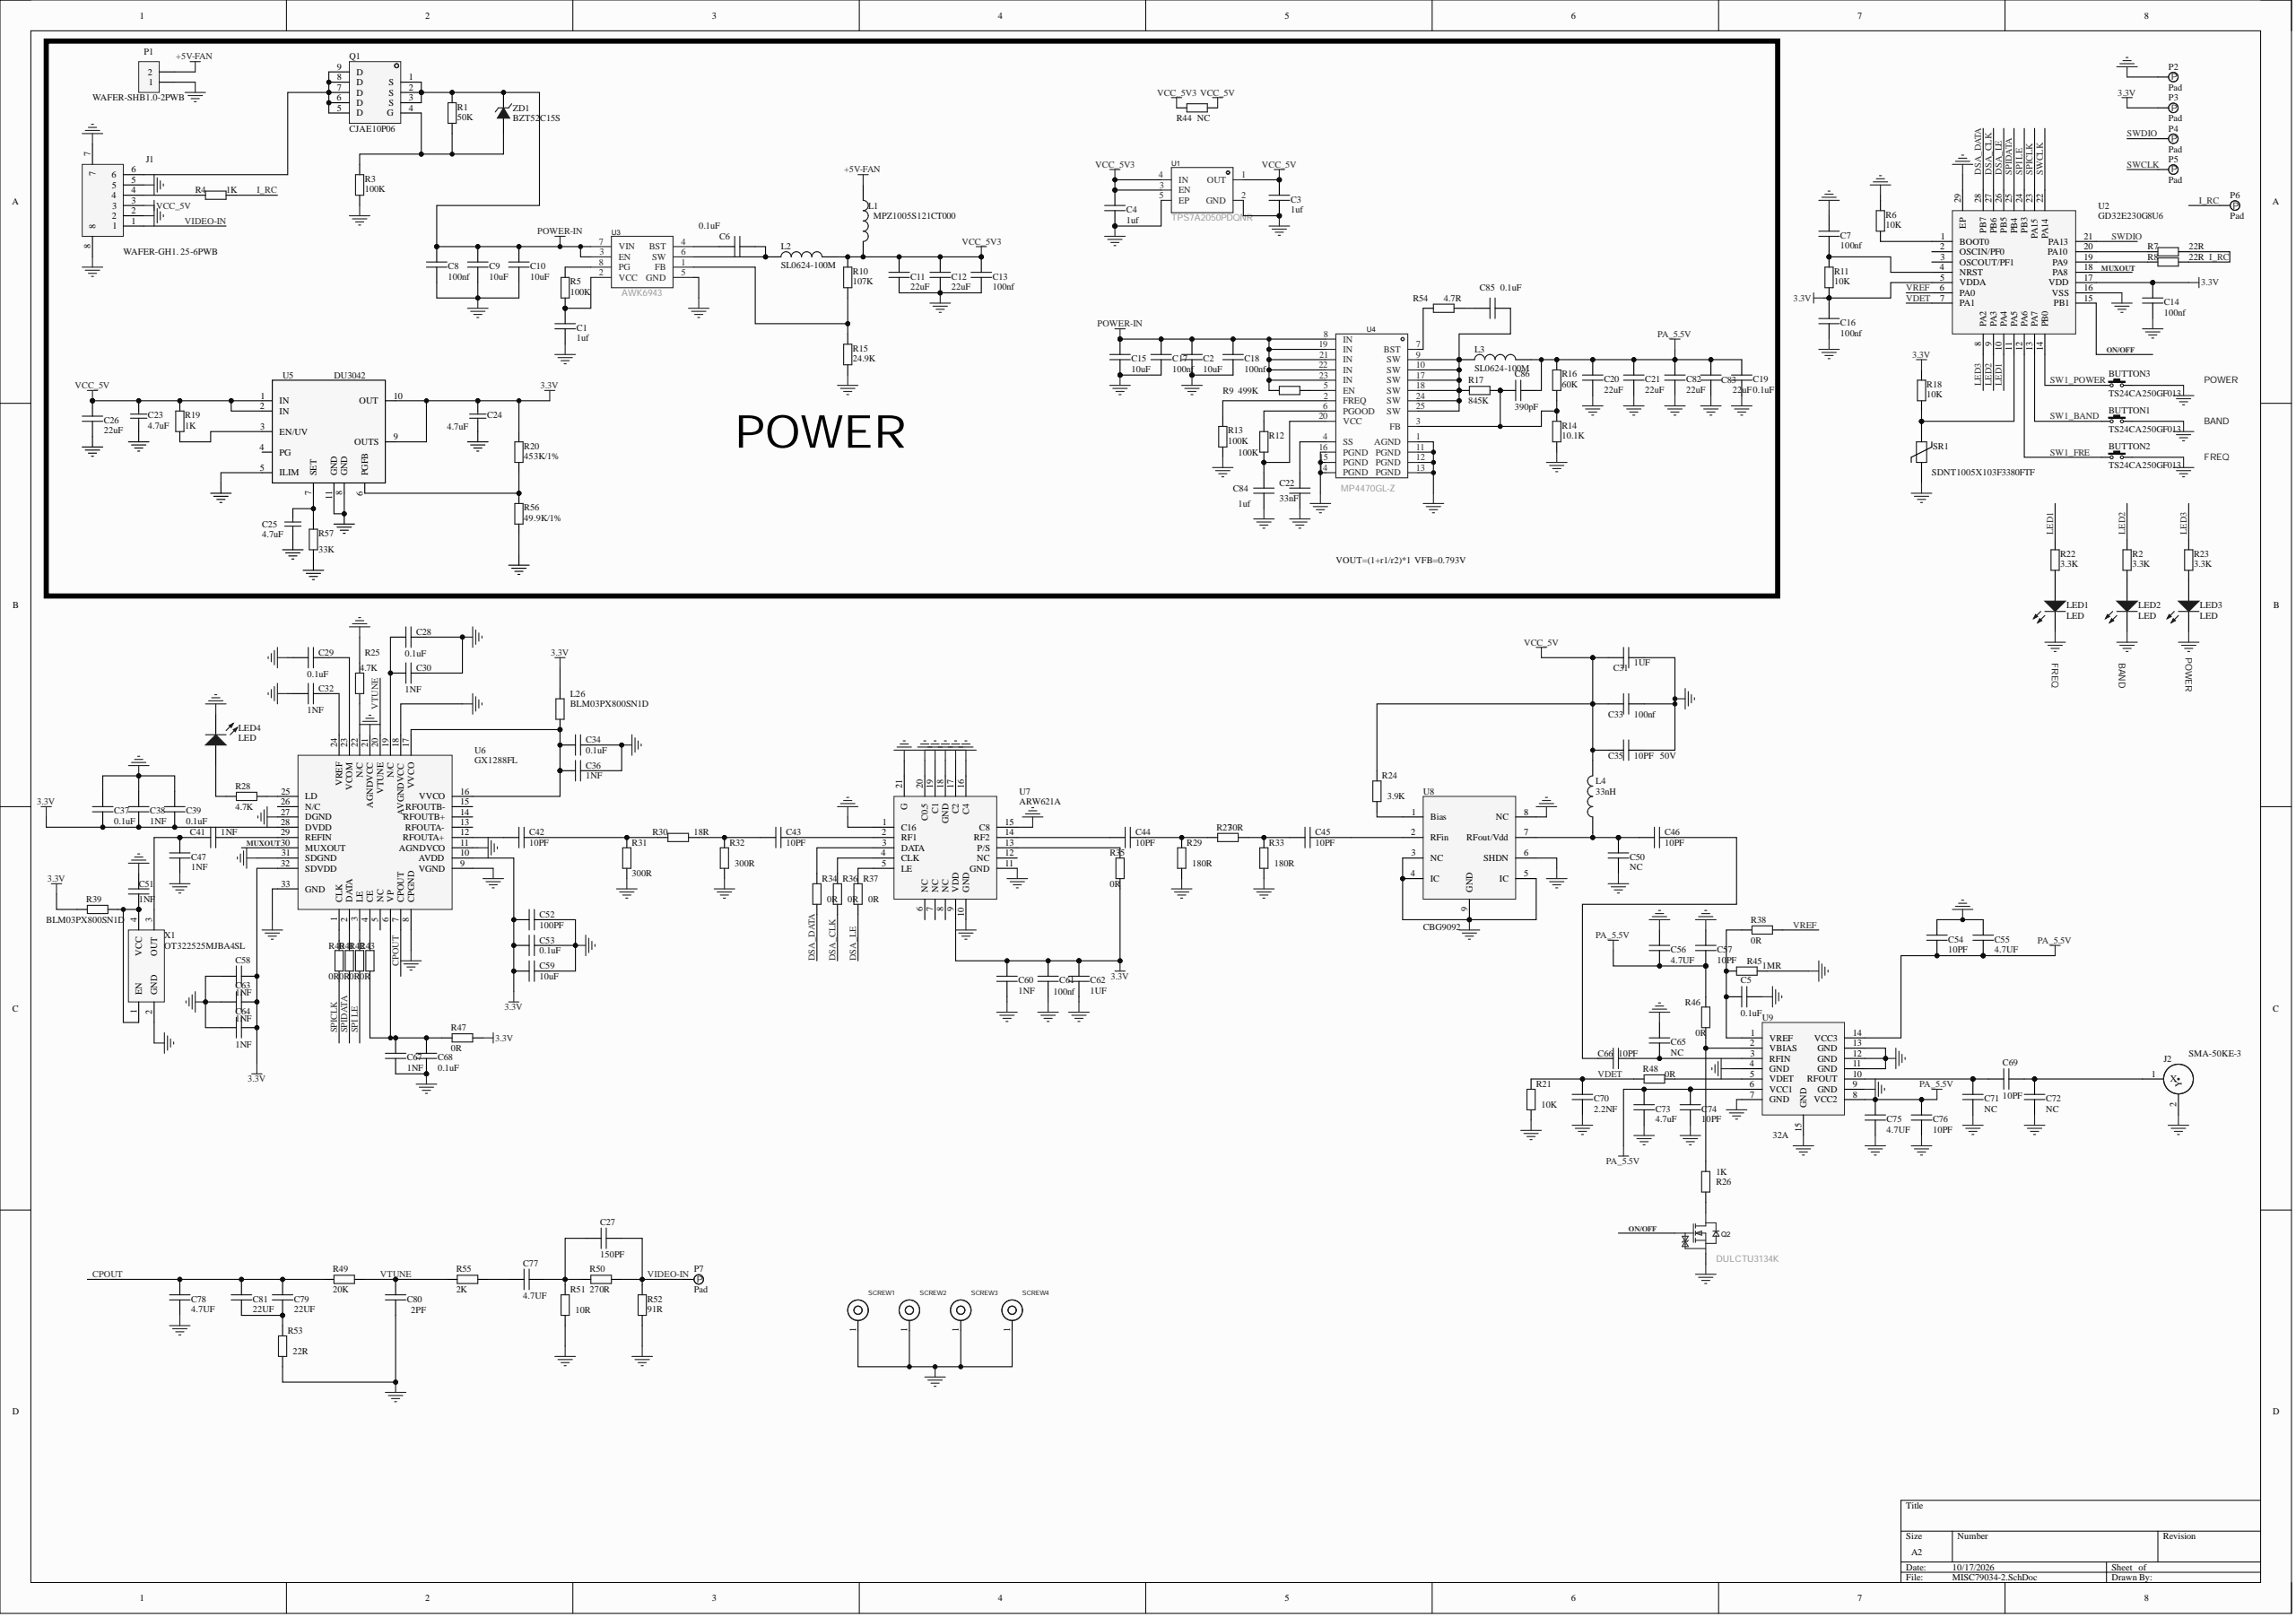Circuit board | Altium Designer | 179 parts | 97 nets
Bill of materials:
Comment,Description,Designator,Footprint,LibRef,Quantity
"TS24CA250GF013","3x6 tact switch","BUTTON1, BUTTON2, BUTTON3","SW-SMD_L4.7-W3.5-P3.35-EH","TSW 3x6","3"
"1uf","","C1, C3, C4, C84","C0603","100nf","4"
"10uF","","C2, C9, C10, C15","C0805","100nf","4"
"0.1uF","","C5, C6, C19, C85","C0402","100nf","4"
"100nf","","C7, C14, C16","C0201","100nf","3"
"100nf","","C8, C13, C17, C18, C33, C61","C0402","100nf","6"
"22uF","","C11, C12, C20, C21, C26, C82, C83","C0603","100nf","7"
"33nF","","C22","C0402","100nf","1"
"4.7uF","Chip capacitor, [NoValue]","C23, C24, C25, C55, C56, C73, C75","C0603","C, 100nf","7"
"150PF","","C27","C0402","100nf","1"
"0.1uF","","C28, C29, C34, C37, C39, C53, C68","C0201","100nf","7"
"1NF","","C30, C32, C36, C38, C41, C47, C51, C58, C63, C64, C67","C0201","100nf","11"
"1UF","","C31, C62","C0402","100nf","2"
"10PF   50V","","C35","C0402","100nf","1"
"10PF","","C42, C43, C44, C45, C46, C54, C57, C66, C69, C74, C76","C0402","100nf","11"
"NC","","C50, C65, C71, C72","C0402","100nf","4"
"100PF","","C52","C0201","100nf","1"
"10uF","","C59","C0402","100nf","1"
"1NF","","C60","C0402","100nf","1"
"2.2NF","","C70","C0402","100nf","1"
"4.7UF","","C77, C78","C0402","100nf","2"
"22UF","","C79, C81","C0402","100nf","2"
"2PF","","C80","C0402","100nf","1"
"390pF","","C86","C0402","100nf","1"
"WAFER-GH1. 25-6PWB","","J1","SMD_6P-P1.25_XUNPU_WAFER-GH1.25-6PWB","WAFER-GH1. 25-6PWB","1"
"SMA-50KE-3","","J2","SMA-FP-945G","SMA-50KE-3","1"
"MPZ1005S121CT000","Color-ring inductor","L1","L0402","L-AL","1"
"SL0624-100M","Color-ring inductor","L2, L3","IND-SMD_L7.1-W6.6","L-AL","2"
"33nH","Color-ring inductor","L4","L0402","L-AL","1"
"BLM03PX800SN1D","Chip resistor","L26, R39","L0201","R","2"
"LED","Light-emitting diode","LED1, LED2, LED3, LED4","LED0402","LED0","4"
"WAFER-SHB1.0-2PWB","2P connector","P1","SMD_2P-WAFER-SHB1.0-2PWB","Header 2","1"
"Pad","","P2, P3, P4, P5, P6, P7","pad","Pad","6"
"CJAE10P06","","Q1","DFN-8_L3.0-W3.0-P0.65-BL_G48N03D3","CJAE10P06","1"
"DULCTU3134K","","Q2","SOT-523-3_L1.6-W0.8-P0.50-LS1.6-BR-1","2N7002T_C5224243","1"
"50K","Chip resistor","R1","R0402","R","1"
"3.3K","Chip resistor","R2, R22, R23","R0402","R","3"
"100K","Chip resistor","R3, R5, R12, R13","R0402","R","4"
"1K","Chip resistor","R4, R19, R26","R0402","R","3"
"10K","Chip resistor","R6, R11, R18","R0201","R","3"
"22R","Chip resistor","R7, R8","R0201","R","2"
"499K","Chip resistor","R9","R0402","R","1"
"107K","Chip resistor","R10","R0402","R","1"
"10.1K","Chip resistor","R14","R0402","R","1"
"24.9K","Chip resistor","R15","R0402","R","1"
"60K","Chip resistor","R16","R0402","R","1"
"845K","Chip resistor","R17","R0402","R","1"
"453K/1%","Chip resistor","R20","R0402","R","1"
"10K","Chip resistor","R21","R0402","R","1"
"3.9K","Chip resistor","R24","R0402","R","1"
"4.7K","Chip resistor","R25, R28","R0201","R","2"
"30R","Chip resistor","R27","R0402","R","1"
"180R","Chip resistor","R29, R33","R0402","R","2"
"18R","Chip resistor","R30","R0402","R","1"
"300R","Chip resistor","R31, R32","R0402","R","2"
"0R","Chip resistor","R34, R35, R36, R37, R38, R46, R48","R0402","R","7"
"0R","Chip resistor","R40, R41, R42, R43, R47","R0201","R","5"
"NC","Chip resistor","R44","R0402","R","1"
"1MR","Chip resistor","R45","R0402","R","1"
"20K","Chip resistor","R49","R0402","R","1"
"270R","Chip resistor","R50","R0402","R","1"
"10R","Chip resistor","R51","R0402","R","1"
"91R","Chip resistor","R52","R0402","R","1"
"22R","Chip resistor","R53","R0402","R","1"
"4.7R","Chip resistor","R54","R1206","R","1"
"2K","Chip resistor","R55","R0402","R","1"
"49.9K/1%","Chip resistor","R56","R0402","R","1"
"33K","Chip resistor","R57","R0402","R","1"
"MARK_4","MARK Symble","SCREW1, SCREW2, SCREW3, SCREW4","M2","MARK_4","4"
"SDNT1005X103F3380FTF","","SR1","R0402","SDNT1005X103F3380FTF","1"
"TPS7A2050PDQNR","","U1","X2SON-4_L1.0-W1.0-P0.65-TL-EP","TPS7A2050PDQNR","1"
"GD32E230G8U6","","U2","QFN-28_L4.0-W4.0-P0.40-BL-EP2.8","GD32E230G8U6","1"
"AWK6943","","U3","QFN-8_L3.0-W3.0-P0.65-BL","TPS54327DDAR","1"
"MP4470GL-Z","","U4","QFN-20_L4.0-W3.0_MP9447GL","MP4470GL-Z","1"
"DU3042","No Description Available","U5","WSON-10_L3.0-W3.0-P0.50-BL-EP","DAC53202RTER","1"
"GX1288FL","","U6","QFN-32_L5.0-W5.0-P0.50","GX1288FL","1"
"ARW621A","","U7","QFN-20_L4.0-W4.0-P0.50-TL-EP2.2","ARW621A","1"
"CBG9092","","U8","CBG9092","CBG9092","1"
"32A","","U9","AU64XX","GCM3527(3.3G-3.8G)","1"
"OT322525MJBA4SL","4-pin active crystal oscillator","X1","SMD3225","XTAL-ACT-4P","1"
"BZT52C15S","5.1V/1W Zener diode","ZD1","SOD-323_L1.7-W1.3-LS2.6-RD","1N4733","1"
Netlist (Protel format):
[
BUTTON1
SW-SMD_L4.7-W3.5-P3.35-EH
TS24CA250GF013



]
[
BUTTON2
SW-SMD_L4.7-W3.5-P3.35-EH
TS24CA250GF013



]
[
BUTTON3
SW-SMD_L4.7-W3.5-P3.35-EH
TS24CA250GF013



]
[
C1
C0603
1uf



]
[
C2
C0805
10uF



]
[
C3
C0603
1uf



]
[
C4
C0603
1uf



]
[
C5
C0402
0.1uF



]
[
C6
C0402
0.1uF



]
[
C7
C0201
100nf



]
[
C8
C0402
100nf



]
[
C9
C0805
10uF



]
[
C10
C0805
10uF



]
[
C11
C0603
22uF



]
[
C12
C0603
22uF



]
[
C13
C0402
100nf



]
[
C14
C0201
100nf



]
[
C15
C0805
10uF



]
[
C16
C0201
100nf



]
[
C17
C0402
100nf



]
[
C18
C0402
100nf



]
[
C19
C0402
0.1uF



]
[
C20
C0603
22uF



]
[
C21
C0603
22uF



]
[
C22
C0402
33nF



]
[
C23
C0603
4.7uF



]
[
C24
C0603
4.7uF



]
[
C25
C0603
4.7uF



]
[
C26
C0603
22uF



]
[
C27
C0402
150PF



]
[
C28
C0201
0.1uF



]
[
C29
C0201
0.1uF



]
[
C30
C0201
1NF



]
[
C31
C0402
1UF



]
[
C32
C0201
1NF



]
[
C33
C0402
100nf



]
[
C34
C0201
0.1uF



]
[
C35
C0402
10PF   50V



]
[
C36
C0201
1NF



]
[
C37
C0201
0.1uF



]
[
C38
C0201
1NF



]
[
C39
C0201
0.1uF



]
[
C41
C0201
1NF



]
[
C42
C0402
10PF



]
[
C43
C0402
10PF



]
[
C44
C0402
10PF



]
[
C45
C0402
10PF



]
[
C46
C0402
10PF



]
[
C47
C0201
1NF



]
[
C50
C0402
NC



]
[
C51
C0201
1NF



]
[
C52
C0201
100PF



]
[
C53
C0201
0.1uF



]
[
C54
C0402
10PF



]
[
C55
C0603
4.7UF



]
[
C56
C0603
4.7UF



]
[
C57
C0402
10PF



]
[
C58
C0201
1NF



]
[
C59
C0402
10uF



]
[
C60
C0402
1NF



]
[
C61
C0402
100nf



]
[
C62
C0402
1UF



]
[
C63
C0201
1NF



]
[
C64
C0201
1NF



]
[
C65
C0402
NC



]
[
C66
C0402
10PF



]
[
C67
C0201
1NF



]
[
C68
C0201
0.1uF



]
[
C69
C0402
10PF



]
[
C70
C0402
2.2NF



]
[
C71
C0402
NC



]
[
C72
C0402
NC



]
[
C73
C0603
4.7uF



]
[
C74
C0402
10PF



]
[
C75
C0603
4.7UF



]
[
C76
C0402
10PF



]
[
C77
C0402
4.7UF



]
[
C78
C0402
4.7UF



]
[
C79
C0402
22UF



]
[
C80
C0402
2PF



]
[
C81
C0402
22UF



]
[
C82
C0603
22uF



]
[
C83
C0603
22uF



]
[
C84
C0603
1uf



]
[
C85
C0402
0.1uF



]
[
C86
C0402
390pF



]
[
J1
SMD_6P-P1.25_XUNPU_WAFER-GH1.25-6PWB
WAFER-GH1. 25-6PWB



]
[
J2
SMA-FP-945G
SMA-50KE-3



]
[
L1
L0402
MPZ1005S121CT000



]
[
L2
IND-SMD_L7.1-W6.6
SL0624-100M



]
[
L3
IND-SMD_L7.1-W6.6
SL0624-100M



]
[
L4
L0402
33nH



]
[
L26
L0201
BLM03PX800SN1D



]
[
LED1
LED0402
LED



]
[
LED2
LED0402
LED



]
[
LED3
LED0402
LED



]
[
LED4
LED0402
LED



]
[
P1
SMD_2P-WAFER-SHB1.0-2PWB
WAFER-SHB1.0-2PWB



]
[
P2
pad
Pad



]
[
P3
pad
Pad



]
[
P4
pad
Pad



]
[
P5
pad
Pad



]
[
P6
PAD
Pad



]
[
P7
PAD
Pad



]
[
Q1
DFN-8_L3.0-W3.0-P0.65-BL_G48N03D3
CJAE10P06



]
[
Q2
SOT-523-3_L1.6-W0.8-P0.50-LS1.6-BR-1
DULCTU3134K



]
[
R1
R0402
50K



]
[
R2
R0402
3.3K



]
[
R3
R0402
100K



]
[
R4
R0402
1K



]
[
R5
R0402
100K



]
[
R6
R0201
10K



]
[
R7
R0201
22R



]
[
R8
R0201
22R



]
[
R9
R0402
499K



]
[
R10
R0402
107K



]
[
R11
R0201
10K



]
[
R12
R0402
100K



]
[
R13
R0402
100K



]
[
R14
R0402
10.1K



]
[
R15
R0402
24.9K



]
[
R16
R0402
60K



]
[
R17
R0402
845K



]
[
R18
R0201
10K



]
[
R19
R0402
1K



]
[
R20
R0402
453K/1%



]
[
R21
R0402
10K



]
[
R22
R0402
3.3K



]
[
R23
R0402
3.3K



]
[
R24
R0402
3.9K



]
[
R25
R0201
4.7K



]
[
R26
R0402
1K



]
[
R27
R0402
30R



]
[
R28
R0201
4.7K



]
[
R29
R0402
180R



]
[
R30
R0402
18R



]
[
R31
R0402
300R



]
[
R32
R0402
300R



]
[
R33
R0402
180R



]
[
R34
R0402
0R



]
[
R35
R0402
0R



]
[
R36
R0402
0R



]
[
R37
R0402
0R



]
[
R38
R0402
0R



]
[
R39
L0201
BLM03PX800SN1D



]
[
R40
R0201
0R



]
[
R41
R0201
0R



]
[
R42
R0201
0R



]
[
R43
R0201
0R



]
[
R44
R0402
NC



]
[
R45
R0402
1MR



]
[
R46
R0402
0R



]
[
R47
R0201
0R



]
[
R48
R0402
0R



]
[
R49
R0402
20K



]
[
R50
R0402
270R



]
[
R51
R0402
10R



]
[
R52
R0402
91R



]
[
R53
R0402
22R



]
[
R54
R1206
4.7R



]
[
R55
R0402
2K



]
[
R56
R0402
49.9K/1%



]
[
R57
R0402
33K



]
[
SCREW1
M2
MARK_4



]
[
SCREW2
M2
MARK_4



]
[
SCREW3
M2
MARK_4



]
[
SCREW4
M2
MARK_4



]
[
SR1
R0402
SDNT1005X103F3380FTF



]
[
U1
X2SON-4_L1.0-W1.0-P0.65-TL-EP
TPS7A2050PDQNR



]
[
U2
QFN-28_L4.0-W4.0-P0.40-BL-EP2.8
GD32E230G8U6



]
[
U3
QFN-8_L3.0-W3.0-P0.65-BL
AWK6943



]
[
U4
QFN-20_L4.0-W3.0_MP9447GL
MP4470GL-Z



]
[
U5
WSON-10_L3.0-W3.0-P0.50-BL-EP
DU3042



]
[
U6
QFN-32_L5.0-W5.0-P0.50
GX1288FL



]
[
U7
QFN-20_L4.0-W4.0-P0.50-TL-EP2.2
ARW621A



]
[
U8
CBG9092
CBG9092



]
[
U9
AU64XX
32A



]
[
X1
SMD3225
OT322525MJBA4SL



]
[
ZD1
SOD-323_L1.7-W1.3-LS2.6-RD
BZT52C15S



]
(
VTUNE
C80-2
R49-2
R55-1
U6-20
)
(
VREF
R38-1
U2-6
)
(
VIDEO-IN
C27-1
J1-1
P7-1
R50-2
R52-1
)
(
VDET
C70-2
R21-1
R48-1
U2-7
)
(
VCC_5V3
C4-1
C11-1
C12-1
C13-1
L1-2
L2-2
R10-1
R44-1
U1-3
U1-4
)
(
VCC_5V
C3-1
C23-2
C26-1
C31-2
C33-2
C35-1
J1-3
L4-2
R19-2
R24-1
R44-2
U1-1
U5-1
U5-2
)
(
SWDIO
P4-1
U2-21
)
(
SWCLK
P5-1
U2-22
)
(
SW1_POWER
BUTTON3-2
U2-14
)
(
SW1_FRE
BUTTON2-2
U2-12
)
(
SW1_BAND
BUTTON1-2
U2-13
)
(
SPIDATA
R41-2
U2-25
)
(
SPICLK
R40-2
U2-23
)
(
SPI LE
R42-2
U2-24
)
(
POWER-IN
C2-1
C8-1
C9-1
C10-1
C15-1
C17-1
C18-1
Q1-1
Q1-2
Q1-3
R1-2
R9-2
U3-3
U3-7
U4-8
U4-19
U4-21
U4-22
U4-23
ZD1-2
)
(
PA_5.5V
C19-2
C20-1
C21-1
C54-1
C55-1
C56-2
C57-2
C73-1
C74-1
C75-1
C76-1
C82-1
C83-1
C86-1
L3-2
R16-1
R46-1
U9-6
U9-8
U9-14
)
(
ON/OFF
Q2-1
U2-15
)
(
NetR54_2
R54-2
U4-7
)
(
NetR48_2
R48-2
U9-5
)
(
NetR43_1
R43-1
U6-4
)
(
NetR42_1
R42-1
U6-3
)
(
NetR41_1
R41-1
U6-2
)
(
NetR40_1
R40-1
U6-1
)
(
NetR37_1
R37-1
U7-5
)
(
NetR36_1
R36-1
U7-4
)
(
NetR35_1
R35-1
U7-13
)
(
NetR34_1
R34-1
U7-3
)
(
NetR28_2
R28-2
U6-25
)
(
NetR26_1
R26-1
R46-2
U9-2
)
(
NetR25_2
R25-2
U6-22
)
(
NetR24_2
R24-2
U8-1
)
(
NetR20_2
R20-2
R56-1
U5-6
)
(
NetR19_1
R19-1
U5-3
)
(
NetR18_2
R18-2
SR1-1
U2-11
)
(
NetR13_1
R13-1
U4-2
)
(
NetR12_1
R12-1
U4-6
)
(
NetR10_2
R10-2
R15-1
U3-1
)
(
NetR9_1
R9-1
U4-5
)
(
NetR8_1
R8-1
U2-19
)
(
NetR7_1
R7-1
U2-20
)
(
NetR6_2
R6-2
U2-1
)
(
NetR5_2
R5-2
U3-8
)
(
NetQ2_3
Q2-3
R26-2
)
(
NetQ1_4
Q1-4
R1-1
R3-2
ZD1-1
)
(
NetLED4_1
LED4-1
R28-1
)
(
NetLED3_1
LED3-1
R23-2
)
(
NetLED2_1
LED2-1
R2-2
)
(
NetLED1_1
LED1-1
R22-2
)
(
NetJ1_6
J1-6
Q1-5
Q1-6
Q1-7
Q1-8
Q1-9
)
(
NetJ1_4
J1-4
R4-1
)
(
NetC86_2
C86-2
R14-1
R16-2
R17-2
U4-3
)
(
NetC85_2
C85-2
L3-1
R17-1
U4-9
U4-10
U4-17
U4-18
U4-24
U4-25
)
(
NetC85_1
C85-1
R54-1
)
(
NetC84_1
C84-1
R12-2
U4-20
)
(
NetC79_1
C79-1
C81-1
R53-1
)
(
NetC77_2
C77-2
R55-2
)
(
NetC69_2
C69-2
C72-2
J2-1
)
(
NetC69_1
C69-1
C71-2
U9-10
)
(
NetC67_1
C67-1
C68-2
R43-2
R47-1
U6-6
)
(
NetC65_1
C65-1
C66-1
U9-3
)
(
NetC51_2
C51-2
R39-2
X1-1
X1-4
)
(
NetC46_2
C46-2
C66-2
)
(
NetC46_1
C46-1
C50-1
L4-1
U8-7
)
(
NetC45_2
C45-2
U8-2
)
(
NetC45_1
C45-1
R27-2
R33-1
)
(
NetC44_2
C44-2
R27-1
R29-1
)
(
NetC44_1
C44-1
U7-14
)
(
NetC43_2
C43-2
U7-2
)
(
NetC43_1
C43-1
R30-2
R32-1
)
(
NetC42_2
C42-2
R30-1
R31-1
)
(
NetC42_1
C42-1
U6-12
)
(
NetC41_2
C41-2
C47-1
X1-3
)
(
NetC41_1
C41-1
U6-29
)
(
NetC34_2
C34-2
C36-1
L26-2
U6-16
U6-17
)
(
NetC32_2
C32-2
U6-24
)
(
NetC29_1
C29-1
U6-23
)
(
NetC28_2
C28-2
C30-1
U6-19
)
(
NetC27_2
C27-2
C77-1
R50-1
R51-1
)
(
NetC25_2
C25-2
R57-2
U5-7
)
(
NetC22_2
C22-2
U4-4
)
(
NetC7_2
C7-2
R11-1
U2-4
)
(
NetC6_2
C6-2
L2-1
U3-6
)
(
NetC6_1
C6-1
U3-4
)
(
NetC5_2
C5-2
R38-2
R45-1
U9-1
)
(
NetC1_1
C1-1
R5-1
U3-2
)
(
MUXOUT
U2-18
U6-30
)
(
LED3
R23-1
U2-8
)
(
LED2
R2-1
U2-9
)
(
LED1
R22-1
U2-10
)
(
I_RC
P6-1
R4-2
R7-2
R8-2
)
(
GND
BUTTON1-1
BUTTON2-1
BUTTON3-1
C1-2
C2-2
C3-2
C4-2
C5-1
C7-1
C8-2
C9-2
C10-2
C11-2
C12-2
C13-2
C14-2
C15-2
C16-2
C17-2
C18-2
C19-1
C20-2
C21-2
C22-1
C23-1
C24-1
C25-1
C26-2
C28-1
C29-2
C30-2
C31-1
C32-1
C33-1
C34-1
C35-2
C36-2
C37-1
C38-2
C39-1
C47-2
C50-2
C51-1
C52-2
C53-1
C54-2
C55-2
C56-1
C57-1
C58-1
C59-1
C60-1
C61-1
C62-1
C63-1
C64-2
C65-2
C67-2
C68-1
C70-1
C71-1
C72-1
C73-2
C74-2
C75-2
C76-2
C78-2
C80-1
C82-2
C83-2
C84-2
J1-2
J1-5
J1-7
J1-8
J2-2
LED1-2
LED2-2
LED3-2
LED4-2
P1-1
P2-1
Q2-2
R3-1
R6-1
R13-2
R14-2
R15-2
R21-2
R25-1
R29-2
R31-2
R32-2
R33-2
R45-2
R51-2
R52-2
R53-2
R56-2
R57-1
SCREW1-1
SCREW2-1
SCREW3-1
SCREW4-1
SR1-2
U1-2
U1-5
U2-16
U2-29
U3-5
U4-1
U4-11
U4-12
U4-13
U4-14
U4-15
U4-16
U5-5
U5-8
U5-11
U6-8
U6-9
U6-11
U6-18
U6-21
U6-27
U6-31
U6-33
U7-1
U7-10
U7-11
U7-15
U7-16
U7-17
U7-18
U7-19
U7-20
U7-21
U8-3
U8-4
U8-5
U8-6
U8-8
U8-9
U9-4
U9-7
U9-9
U9-11
U9-12
U9-13
U9-15
X1-2
)
(
DSA_LE
R37-2
U2-26
)
(
DSA_DATA
R34-2
U2-28
)
(
DSA_CLK
R36-2
U2-27
)
(
CPOUT
C78-1
C79-2
C81-2
R49-1
U6-7
)
(
+5V-FAN
L1-1
P1-2
)
(
3.3V
C14-1
C16-1
C24-2
C37-2
C38-1
C39-2
C52-1
C53-2
C58-2
C59-2
C60-2
C61-2
C62-2
C63-2
C64-1
L26-1
P3-1
R11-2
R18-1
R20-1
R35-2
R39-1
R47-2
U2-5
U2-17
U5-9
U5-10
U6-10
U6-28
U6-32
U7-9
)